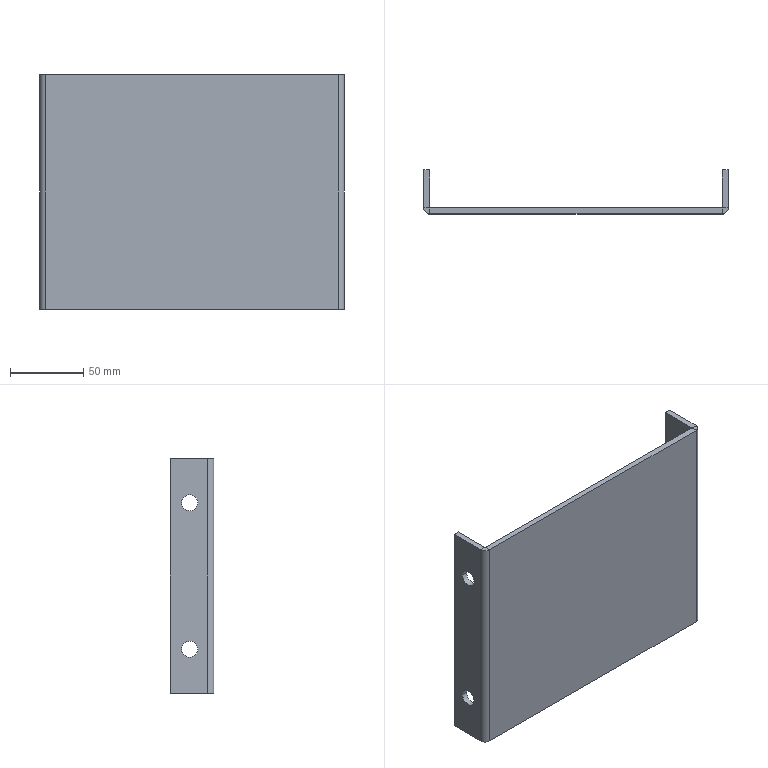Part | SolidWorks | features FlatPattern 1, ICE 1, SMBaseFlange 1, SheetMetal 1 | 1 solid | 30 faces | box 208 x 30 x 160 mm | volume 163671 mm3 | plane 18 | cylinder 12 | commonest cylinder face diameters 11 x8 0.4 x2 8.4 x2
STEP:
#1=CARTESIAN_POINT('',(100.,22.,50.));
#2=VERTEX_POINT('',#1);
#3=CARTESIAN_POINT('',(100.,11.,50.));
#4=VERTEX_POINT('',#3);
#5=CARTESIAN_POINT('',(100.,16.5,50.));
#6=DIRECTION('',(-1.,0.,0.));
#7=DIRECTION('',(0.,-1.,0.));
#8=AXIS2_PLACEMENT_3D('',#5,#6,#7);
#9=CIRCLE('',#8,5.5);
#10=EDGE_CURVE('',#2,#4,#9,.T.);
#11=ORIENTED_EDGE('',*,*,#10,.T.);
#12=CARTESIAN_POINT('',(104.,11.,50.));
#13=VERTEX_POINT('',#12);
#14=CARTESIAN_POINT('',(-104.,11.,50.));
#15=DIRECTION('',(1.,0.,0.));
#16=VECTOR('',#15,1000.);
#17=LINE('',#14,#16);
#18=EDGE_CURVE('',#4,#13,#17,.T.);
#19=ORIENTED_EDGE('',*,*,#18,.T.);
#20=CARTESIAN_POINT('',(104.,22.,50.));
#21=VERTEX_POINT('',#20);
#22=CARTESIAN_POINT('',(104.,16.5,50.));
#23=DIRECTION('',(-1.,0.,0.));
#24=DIRECTION('',(0.,-1.,0.));
#25=AXIS2_PLACEMENT_3D('',#22,#23,#24);
#26=CIRCLE('',#25,5.5);
#27=EDGE_CURVE('',#21,#13,#26,.T.);
#28=ORIENTED_EDGE('',*,*,#27,.F.);
#29=CARTESIAN_POINT('',(-104.,22.,50.));
#30=DIRECTION('',(1.,0.,0.));
#31=VECTOR('',#30,1000.);
#32=LINE('',#29,#31);
#33=EDGE_CURVE('',#2,#21,#32,.T.);
#34=ORIENTED_EDGE('',*,*,#33,.F.);
#35=EDGE_LOOP('',(#11,#19,#28,#34));
#36=FACE_OUTER_BOUND('',#35,.T.);
#37=CARTESIAN_POINT('',(-104.,16.5,50.));
#38=DIRECTION('',(1.,0.,0.));
#39=DIRECTION('',(0.,1.,0.));
#40=AXIS2_PLACEMENT_3D('',#37,#38,#39);
#41=CYLINDRICAL_SURFACE('',#40,5.5);
#42=ADVANCED_FACE('',(#36),#41,.F.);
#43=CARTESIAN_POINT('',(100.,22.,-50.));
#44=VERTEX_POINT('',#43);
#45=CARTESIAN_POINT('',(100.,11.,-50.));
#46=VERTEX_POINT('',#45);
#47=CARTESIAN_POINT('',(100.,16.5,-50.));
#48=DIRECTION('',(-1.,0.,0.));
#49=DIRECTION('',(0.,-1.,0.));
#50=AXIS2_PLACEMENT_3D('',#47,#48,#49);
#51=CIRCLE('',#50,5.5);
#52=EDGE_CURVE('',#44,#46,#51,.T.);
#53=ORIENTED_EDGE('',*,*,#52,.T.);
#54=CARTESIAN_POINT('',(104.,11.,-50.));
#55=VERTEX_POINT('',#54);
#56=CARTESIAN_POINT('',(-104.,11.,-50.));
#57=DIRECTION('',(1.,0.,0.));
#58=VECTOR('',#57,1000.);
#59=LINE('',#56,#58);
#60=EDGE_CURVE('',#46,#55,#59,.T.);
#61=ORIENTED_EDGE('',*,*,#60,.T.);
#62=CARTESIAN_POINT('',(104.,22.,-50.));
#63=VERTEX_POINT('',#62);
#64=CARTESIAN_POINT('',(104.,16.5,-50.));
#65=DIRECTION('',(-1.,0.,0.));
#66=DIRECTION('',(0.,-1.,0.));
#67=AXIS2_PLACEMENT_3D('',#64,#65,#66);
#68=CIRCLE('',#67,5.5);
#69=EDGE_CURVE('',#63,#55,#68,.T.);
#70=ORIENTED_EDGE('',*,*,#69,.F.);
#71=CARTESIAN_POINT('',(-104.,22.,-50.));
#72=DIRECTION('',(1.,0.,0.));
#73=VECTOR('',#72,1000.);
#74=LINE('',#71,#73);
#75=EDGE_CURVE('',#44,#63,#74,.T.);
#76=ORIENTED_EDGE('',*,*,#75,.F.);
#77=EDGE_LOOP('',(#53,#61,#70,#76));
#78=FACE_OUTER_BOUND('',#77,.T.);
#79=CARTESIAN_POINT('',(-104.,16.5,-50.));
#80=DIRECTION('',(1.,0.,0.));
#81=DIRECTION('',(0.,1.,0.));
#82=AXIS2_PLACEMENT_3D('',#79,#80,#81);
#83=CYLINDRICAL_SURFACE('',#82,5.5);
#84=ADVANCED_FACE('',(#78),#83,.F.);
#85=CARTESIAN_POINT('',(-104.,11.,50.));
#86=VERTEX_POINT('',#85);
#87=CARTESIAN_POINT('',(-104.,22.,50.));
#88=VERTEX_POINT('',#87);
#89=CARTESIAN_POINT('',(-104.,16.5,50.));
#90=DIRECTION('',(1.,0.,0.));
#91=DIRECTION('',(0.,1.,0.));
#92=AXIS2_PLACEMENT_3D('',#89,#90,#91);
#93=CIRCLE('',#92,5.5);
#94=EDGE_CURVE('',#86,#88,#93,.T.);
#95=ORIENTED_EDGE('',*,*,#94,.F.);
#96=CARTESIAN_POINT('',(-100.,11.,50.));
#97=VERTEX_POINT('',#96);
#98=CARTESIAN_POINT('',(-104.,11.,50.));
#99=DIRECTION('',(1.,0.,0.));
#100=VECTOR('',#99,1000.);
#101=LINE('',#98,#100);
#102=EDGE_CURVE('',#86,#97,#101,.T.);
#103=ORIENTED_EDGE('',*,*,#102,.T.);
#104=CARTESIAN_POINT('',(-100.,22.,50.));
#105=VERTEX_POINT('',#104);
#106=CARTESIAN_POINT('',(-100.,16.5,50.));
#107=DIRECTION('',(1.,0.,0.));
#108=DIRECTION('',(0.,1.,0.));
#109=AXIS2_PLACEMENT_3D('',#106,#107,#108);
#110=CIRCLE('',#109,5.5);
#111=EDGE_CURVE('',#97,#105,#110,.T.);
#112=ORIENTED_EDGE('',*,*,#111,.T.);
#113=CARTESIAN_POINT('',(-104.,22.,50.));
#114=DIRECTION('',(1.,0.,0.));
#115=VECTOR('',#114,1000.);
#116=LINE('',#113,#115);
#117=EDGE_CURVE('',#88,#105,#116,.T.);
#118=ORIENTED_EDGE('',*,*,#117,.F.);
#119=EDGE_LOOP('',(#95,#103,#112,#118));
#120=FACE_OUTER_BOUND('',#119,.T.);
#121=CARTESIAN_POINT('',(-104.,16.5,50.));
#122=DIRECTION('',(1.,0.,0.));
#123=DIRECTION('',(0.,1.,0.));
#124=AXIS2_PLACEMENT_3D('',#121,#122,#123);
#125=CYLINDRICAL_SURFACE('',#124,5.5);
#126=ADVANCED_FACE('',(#120),#125,.F.);
#127=CARTESIAN_POINT('',(-104.,11.,-50.));
#128=VERTEX_POINT('',#127);
#129=CARTESIAN_POINT('',(-104.,22.,-50.));
#130=VERTEX_POINT('',#129);
#131=CARTESIAN_POINT('',(-104.,16.5,-50.));
#132=DIRECTION('',(1.,0.,0.));
#133=DIRECTION('',(0.,1.,0.));
#134=AXIS2_PLACEMENT_3D('',#131,#132,#133);
#135=CIRCLE('',#134,5.5);
#136=EDGE_CURVE('',#128,#130,#135,.T.);
#137=ORIENTED_EDGE('',*,*,#136,.F.);
#138=CARTESIAN_POINT('',(-100.,11.,-50.));
#139=VERTEX_POINT('',#138);
#140=CARTESIAN_POINT('',(-104.,11.,-50.));
#141=DIRECTION('',(1.,0.,0.));
#142=VECTOR('',#141,1000.);
#143=LINE('',#140,#142);
#144=EDGE_CURVE('',#128,#139,#143,.T.);
#145=ORIENTED_EDGE('',*,*,#144,.T.);
#146=CARTESIAN_POINT('',(-100.,22.,-50.));
#147=VERTEX_POINT('',#146);
#148=CARTESIAN_POINT('',(-100.,16.5,-50.));
#149=DIRECTION('',(1.,0.,0.));
#150=DIRECTION('',(0.,1.,0.));
#151=AXIS2_PLACEMENT_3D('',#148,#149,#150);
#152=CIRCLE('',#151,5.5);
#153=EDGE_CURVE('',#139,#147,#152,.T.);
#154=ORIENTED_EDGE('',*,*,#153,.T.);
#155=CARTESIAN_POINT('',(-104.,22.,-50.));
#156=DIRECTION('',(1.,0.,0.));
#157=VECTOR('',#156,1000.);
#158=LINE('',#155,#157);
#159=EDGE_CURVE('',#130,#147,#158,.T.);
#160=ORIENTED_EDGE('',*,*,#159,.F.);
#161=EDGE_LOOP('',(#137,#145,#154,#160));
#162=FACE_OUTER_BOUND('',#161,.T.);
#163=CARTESIAN_POINT('',(-104.,16.5,-50.));
#164=DIRECTION('',(1.,0.,0.));
#165=DIRECTION('',(0.,1.,0.));
#166=AXIS2_PLACEMENT_3D('',#163,#164,#165);
#167=CYLINDRICAL_SURFACE('',#166,5.5);
#168=ADVANCED_FACE('',(#162),#167,.F.);
#169=CARTESIAN_POINT('',(-104.,4.2,80.));
#170=VERTEX_POINT('',#169);
#171=CARTESIAN_POINT('',(-100.,4.2,80.));
#172=VERTEX_POINT('',#171);
#173=CARTESIAN_POINT('',(-104.,4.2,80.));
#174=DIRECTION('',(1.,0.,0.));
#175=VECTOR('',#174,1000.);
#176=LINE('',#173,#175);
#177=EDGE_CURVE('',#170,#172,#176,.T.);
#178=ORIENTED_EDGE('',*,*,#177,.F.);
#179=CARTESIAN_POINT('',(-99.8,0.,80.));
#180=VERTEX_POINT('',#179);
#181=CARTESIAN_POINT('',(-99.8,4.2,80.));
#182=DIRECTION('',(0.,0.,1.));
#183=DIRECTION('',(-1.,0.,0.));
#184=AXIS2_PLACEMENT_3D('',#181,#182,#183);
#185=CIRCLE('',#184,4.2);
#186=EDGE_CURVE('',#170,#180,#185,.T.);
#187=ORIENTED_EDGE('',*,*,#186,.T.);
#188=CARTESIAN_POINT('',(-99.8,4.,80.));
#189=VERTEX_POINT('',#188);
#190=CARTESIAN_POINT('',(-99.8,4.,80.));
#191=DIRECTION('',(0.,-1.,0.));
#192=VECTOR('',#191,1000.);
#193=LINE('',#190,#192);
#194=EDGE_CURVE('',#189,#180,#193,.T.);
#195=ORIENTED_EDGE('',*,*,#194,.F.);
#196=CARTESIAN_POINT('',(-99.8,4.2,80.));
#197=DIRECTION('',(0.,0.,1.));
#198=DIRECTION('',(1.,0.,0.));
#199=AXIS2_PLACEMENT_3D('',#196,#197,#198);
#200=CIRCLE('',#199,0.2);
#201=EDGE_CURVE('',#172,#189,#200,.T.);
#202=ORIENTED_EDGE('',*,*,#201,.F.);
#203=EDGE_LOOP('',(#178,#187,#195,#202));
#204=FACE_OUTER_BOUND('',#203,.T.);
#205=CARTESIAN_POINT('',(-104.,4.2,80.));
#206=DIRECTION('',(0.,0.,1.));
#207=DIRECTION('',(1.,0.,0.));
#208=AXIS2_PLACEMENT_3D('',#205,#206,#207);
#209=PLANE('',#208);
#210=ADVANCED_FACE('',(#204),#209,.T.);
#211=CARTESIAN_POINT('',(-104.,30.,80.));
#212=VERTEX_POINT('',#211);
#213=CARTESIAN_POINT('',(-104.,30.,80.));
#214=DIRECTION('',(0.,-1.,0.));
#215=VECTOR('',#214,1000.);
#216=LINE('',#213,#215);
#217=EDGE_CURVE('',#212,#170,#216,.T.);
#218=ORIENTED_EDGE('',*,*,#217,.T.);
#219=ORIENTED_EDGE('',*,*,#177,.T.);
#220=CARTESIAN_POINT('',(-100.,30.,80.));
#221=VERTEX_POINT('',#220);
#222=CARTESIAN_POINT('',(-100.,30.,80.));
#223=DIRECTION('',(0.,-1.,0.));
#224=VECTOR('',#223,1000.);
#225=LINE('',#222,#224);
#226=EDGE_CURVE('',#221,#172,#225,.T.);
#227=ORIENTED_EDGE('',*,*,#226,.F.);
#228=CARTESIAN_POINT('',(-104.,30.,80.));
#229=DIRECTION('',(1.,0.,0.));
#230=VECTOR('',#229,1000.);
#231=LINE('',#228,#230);
#232=EDGE_CURVE('',#212,#221,#231,.T.);
#233=ORIENTED_EDGE('',*,*,#232,.F.);
#234=EDGE_LOOP('',(#218,#219,#227,#233));
#235=FACE_OUTER_BOUND('',#234,.T.);
#236=CARTESIAN_POINT('',(-99.8,4.,80.));
#237=DIRECTION('',(0.,0.,1.));
#238=DIRECTION('',(1.,0.,0.));
#239=AXIS2_PLACEMENT_3D('',#236,#237,#238);
#240=PLANE('',#239);
#241=ADVANCED_FACE('',(#235),#240,.T.);
#242=CARTESIAN_POINT('',(-99.8,0.,-80.));
#243=VERTEX_POINT('',#242);
#244=CARTESIAN_POINT('',(-99.8,4.,-80.));
#245=VERTEX_POINT('',#244);
#246=CARTESIAN_POINT('',(-99.8,0.,-80.));
#247=DIRECTION('',(0.,1.,0.));
#248=VECTOR('',#247,1000.);
#249=LINE('',#246,#248);
#250=EDGE_CURVE('',#243,#245,#249,.T.);
#251=ORIENTED_EDGE('',*,*,#250,.F.);
#252=CARTESIAN_POINT('',(-104.,4.2,-80.));
#253=VERTEX_POINT('',#252);
#254=CARTESIAN_POINT('',(-99.8,4.2,-80.));
#255=DIRECTION('',(0.,0.,1.));
#256=DIRECTION('',(-1.,0.,0.));
#257=AXIS2_PLACEMENT_3D('',#254,#255,#256);
#258=CIRCLE('',#257,4.2);
#259=EDGE_CURVE('',#253,#243,#258,.T.);
#260=ORIENTED_EDGE('',*,*,#259,.F.);
#261=CARTESIAN_POINT('',(-100.,4.2,-80.));
#262=VERTEX_POINT('',#261);
#263=CARTESIAN_POINT('',(-100.,4.2,-80.));
#264=DIRECTION('',(-1.,0.,0.));
#265=VECTOR('',#264,1000.);
#266=LINE('',#263,#265);
#267=EDGE_CURVE('',#262,#253,#266,.T.);
#268=ORIENTED_EDGE('',*,*,#267,.F.);
#269=CARTESIAN_POINT('',(-99.8,4.2,-80.));
#270=DIRECTION('',(0.,0.,1.));
#271=DIRECTION('',(1.,0.,0.));
#272=AXIS2_PLACEMENT_3D('',#269,#270,#271);
#273=CIRCLE('',#272,0.2);
#274=EDGE_CURVE('',#262,#245,#273,.T.);
#275=ORIENTED_EDGE('',*,*,#274,.T.);
#276=EDGE_LOOP('',(#251,#260,#268,#275));
#277=FACE_OUTER_BOUND('',#276,.T.);
#278=CARTESIAN_POINT('',(-99.8,0.,-80.));
#279=DIRECTION('',(0.,0.,-1.));
#280=DIRECTION('',(-1.,0.,0.));
#281=AXIS2_PLACEMENT_3D('',#278,#279,#280);
#282=PLANE('',#281);
#283=ADVANCED_FACE('',(#277),#282,.T.);
#284=CARTESIAN_POINT('',(99.8,0.,-80.));
#285=VERTEX_POINT('',#284);
#286=CARTESIAN_POINT('',(-104.,0.,-80.));
#287=DIRECTION('',(1.,0.,0.));
#288=VECTOR('',#287,1000.);
#289=LINE('',#286,#288);
#290=EDGE_CURVE('',#243,#285,#289,.T.);
#291=ORIENTED_EDGE('',*,*,#290,.F.);
#292=ORIENTED_EDGE('',*,*,#250,.T.);
#293=CARTESIAN_POINT('',(99.8,4.,-80.));
#294=VERTEX_POINT('',#293);
#295=CARTESIAN_POINT('',(-104.,4.,-80.));
#296=DIRECTION('',(1.,0.,0.));
#297=VECTOR('',#296,1000.);
#298=LINE('',#295,#297);
#299=EDGE_CURVE('',#245,#294,#298,.T.);
#300=ORIENTED_EDGE('',*,*,#299,.T.);
#301=CARTESIAN_POINT('',(99.8,4.,-80.));
#302=DIRECTION('',(0.,-1.,0.));
#303=VECTOR('',#302,1000.);
#304=LINE('',#301,#303);
#305=EDGE_CURVE('',#294,#285,#304,.T.);
#306=ORIENTED_EDGE('',*,*,#305,.T.);
#307=EDGE_LOOP('',(#291,#292,#300,#306));
#308=FACE_OUTER_BOUND('',#307,.T.);
#309=CARTESIAN_POINT('',(-100.,4.2,-80.));
#310=DIRECTION('',(0.,0.,-1.));
#311=DIRECTION('',(-1.,0.,0.));
#312=AXIS2_PLACEMENT_3D('',#309,#310,#311);
#313=PLANE('',#312);
#314=ADVANCED_FACE('',(#308),#313,.T.);
#315=CARTESIAN_POINT('',(99.8,0.,80.));
#316=VERTEX_POINT('',#315);
#317=CARTESIAN_POINT('',(99.8,4.,80.));
#318=VERTEX_POINT('',#317);
#319=CARTESIAN_POINT('',(99.8,0.,80.));
#320=DIRECTION('',(0.,1.,0.));
#321=VECTOR('',#320,1000.);
#322=LINE('',#319,#321);
#323=EDGE_CURVE('',#316,#318,#322,.T.);
#324=ORIENTED_EDGE('',*,*,#323,.F.);
#325=CARTESIAN_POINT('',(104.,4.2,80.));
#326=VERTEX_POINT('',#325);
#327=CARTESIAN_POINT('',(99.8,4.2,80.));
#328=DIRECTION('',(0.,0.,1.));
#329=DIRECTION('',(-1.,0.,0.));
#330=AXIS2_PLACEMENT_3D('',#327,#328,#329);
#331=CIRCLE('',#330,4.2);
#332=EDGE_CURVE('',#316,#326,#331,.T.);
#333=ORIENTED_EDGE('',*,*,#332,.T.);
#334=CARTESIAN_POINT('',(100.,4.2,80.));
#335=VERTEX_POINT('',#334);
#336=CARTESIAN_POINT('',(100.,4.2,80.));
#337=DIRECTION('',(1.,0.,0.));
#338=VECTOR('',#337,1000.);
#339=LINE('',#336,#338);
#340=EDGE_CURVE('',#335,#326,#339,.T.);
#341=ORIENTED_EDGE('',*,*,#340,.F.);
#342=CARTESIAN_POINT('',(99.8,4.2,80.));
#343=DIRECTION('',(0.,0.,1.));
#344=DIRECTION('',(1.,0.,0.));
#345=AXIS2_PLACEMENT_3D('',#342,#343,#344);
#346=CIRCLE('',#345,0.2);
#347=EDGE_CURVE('',#318,#335,#346,.T.);
#348=ORIENTED_EDGE('',*,*,#347,.F.);
#349=EDGE_LOOP('',(#324,#333,#341,#348));
#350=FACE_OUTER_BOUND('',#349,.T.);
#351=CARTESIAN_POINT('',(99.8,0.,80.));
#352=DIRECTION('',(0.,0.,1.));
#353=DIRECTION('',(1.,0.,0.));
#354=AXIS2_PLACEMENT_3D('',#351,#352,#353);
#355=PLANE('',#354);
#356=ADVANCED_FACE('',(#350),#355,.T.);
#357=CARTESIAN_POINT('',(-104.,0.,80.));
#358=DIRECTION('',(1.,0.,0.));
#359=VECTOR('',#358,1000.);
#360=LINE('',#357,#359);
#361=EDGE_CURVE('',#180,#316,#360,.T.);
#362=ORIENTED_EDGE('',*,*,#361,.T.);
#363=ORIENTED_EDGE('',*,*,#323,.T.);
#364=CARTESIAN_POINT('',(-104.,4.,80.));
#365=DIRECTION('',(1.,0.,0.));
#366=VECTOR('',#365,1000.);
#367=LINE('',#364,#366);
#368=EDGE_CURVE('',#189,#318,#367,.T.);
#369=ORIENTED_EDGE('',*,*,#368,.F.);
#370=ORIENTED_EDGE('',*,*,#194,.T.);
#371=EDGE_LOOP('',(#362,#363,#369,#370));
#372=FACE_OUTER_BOUND('',#371,.T.);
#373=CARTESIAN_POINT('',(100.,4.2,80.));
#374=DIRECTION('',(0.,0.,1.));
#375=DIRECTION('',(1.,0.,0.));
#376=AXIS2_PLACEMENT_3D('',#373,#374,#375);
#377=PLANE('',#376);
#378=ADVANCED_FACE('',(#372),#377,.T.);
#379=CARTESIAN_POINT('',(104.,4.2,-80.));
#380=VERTEX_POINT('',#379);
#381=CARTESIAN_POINT('',(100.,4.2,-80.));
#382=VERTEX_POINT('',#381);
#383=CARTESIAN_POINT('',(104.,4.2,-80.));
#384=DIRECTION('',(-1.,0.,0.));
#385=VECTOR('',#384,1000.);
#386=LINE('',#383,#385);
#387=EDGE_CURVE('',#380,#382,#386,.T.);
#388=ORIENTED_EDGE('',*,*,#387,.F.);
#389=CARTESIAN_POINT('',(99.8,4.2,-80.));
#390=DIRECTION('',(0.,0.,1.));
#391=DIRECTION('',(-1.,0.,0.));
#392=AXIS2_PLACEMENT_3D('',#389,#390,#391);
#393=CIRCLE('',#392,4.2);
#394=EDGE_CURVE('',#285,#380,#393,.T.);
#395=ORIENTED_EDGE('',*,*,#394,.F.);
#396=ORIENTED_EDGE('',*,*,#305,.F.);
#397=CARTESIAN_POINT('',(99.8,4.2,-80.));
#398=DIRECTION('',(0.,0.,1.));
#399=DIRECTION('',(1.,0.,0.));
#400=AXIS2_PLACEMENT_3D('',#397,#398,#399);
#401=CIRCLE('',#400,0.2);
#402=EDGE_CURVE('',#294,#382,#401,.T.);
#403=ORIENTED_EDGE('',*,*,#402,.T.);
#404=EDGE_LOOP('',(#388,#395,#396,#403));
#405=FACE_OUTER_BOUND('',#404,.T.);
#406=CARTESIAN_POINT('',(104.,4.2,-80.));
#407=DIRECTION('',(0.,0.,-1.));
#408=DIRECTION('',(-1.,0.,0.));
#409=AXIS2_PLACEMENT_3D('',#406,#407,#408);
#410=PLANE('',#409);
#411=ADVANCED_FACE('',(#405),#410,.T.);
#412=CARTESIAN_POINT('',(104.,30.,-80.));
#413=VERTEX_POINT('',#412);
#414=CARTESIAN_POINT('',(104.,0.,-80.));
#415=DIRECTION('',(0.,1.,0.));
#416=VECTOR('',#415,1000.);
#417=LINE('',#414,#416);
#418=EDGE_CURVE('',#380,#413,#417,.T.);
#419=ORIENTED_EDGE('',*,*,#418,.F.);
#420=ORIENTED_EDGE('',*,*,#387,.T.);
#421=CARTESIAN_POINT('',(100.,30.,-80.));
#422=VERTEX_POINT('',#421);
#423=CARTESIAN_POINT('',(100.,0.,-80.));
#424=DIRECTION('',(0.,1.,0.));
#425=VECTOR('',#424,1000.);
#426=LINE('',#423,#425);
#427=EDGE_CURVE('',#382,#422,#426,.T.);
#428=ORIENTED_EDGE('',*,*,#427,.T.);
#429=CARTESIAN_POINT('',(100.,30.,-80.));
#430=DIRECTION('',(1.,0.,0.));
#431=VECTOR('',#430,1000.);
#432=LINE('',#429,#431);
#433=EDGE_CURVE('',#422,#413,#432,.T.);
#434=ORIENTED_EDGE('',*,*,#433,.T.);
#435=EDGE_LOOP('',(#419,#420,#428,#434));
#436=FACE_OUTER_BOUND('',#435,.T.);
#437=CARTESIAN_POINT('',(99.8,4.,-80.));
#438=DIRECTION('',(0.,0.,-1.));
#439=DIRECTION('',(-1.,0.,0.));
#440=AXIS2_PLACEMENT_3D('',#437,#438,#439);
#441=PLANE('',#440);
#442=ADVANCED_FACE('',(#436),#441,.T.);
#443=ORIENTED_EDGE('',*,*,#27,.T.);
#444=CARTESIAN_POINT('',(104.,16.5,50.));
#445=DIRECTION('',(-1.,0.,0.));
#446=DIRECTION('',(0.,-1.,0.));
#447=AXIS2_PLACEMENT_3D('',#444,#445,#446);
#448=CIRCLE('',#447,5.5);
#449=EDGE_CURVE('',#13,#21,#448,.T.);
#450=ORIENTED_EDGE('',*,*,#449,.T.);
#451=EDGE_LOOP('',(#443,#450));
#452=FACE_BOUND('',#451,.T.);
#453=ORIENTED_EDGE('',*,*,#69,.T.);
#454=CARTESIAN_POINT('',(104.,16.5,-50.));
#455=DIRECTION('',(-1.,0.,0.));
#456=DIRECTION('',(0.,-1.,0.));
#457=AXIS2_PLACEMENT_3D('',#454,#455,#456);
#458=CIRCLE('',#457,5.5);
#459=EDGE_CURVE('',#55,#63,#458,.T.);
#460=ORIENTED_EDGE('',*,*,#459,.T.);
#461=EDGE_LOOP('',(#453,#460));
#462=FACE_BOUND('',#461,.T.);
#463=ORIENTED_EDGE('',*,*,#418,.T.);
#464=CARTESIAN_POINT('',(104.,30.,80.));
#465=VERTEX_POINT('',#464);
#466=CARTESIAN_POINT('',(104.,30.,80.));
#467=DIRECTION('',(0.,0.,-1.));
#468=VECTOR('',#467,1000.);
#469=LINE('',#466,#468);
#470=EDGE_CURVE('',#465,#413,#469,.T.);
#471=ORIENTED_EDGE('',*,*,#470,.F.);
#472=CARTESIAN_POINT('',(104.,0.,80.));
#473=DIRECTION('',(0.,1.,0.));
#474=VECTOR('',#473,1000.);
#475=LINE('',#472,#474);
#476=EDGE_CURVE('',#326,#465,#475,.T.);
#477=ORIENTED_EDGE('',*,*,#476,.F.);
#478=CARTESIAN_POINT('',(104.,4.2,80.));
#479=DIRECTION('',(0.,0.,-1.));
#480=VECTOR('',#479,1000.);
#481=LINE('',#478,#480);
#482=EDGE_CURVE('',#326,#380,#481,.T.);
#483=ORIENTED_EDGE('',*,*,#482,.T.);
#484=EDGE_LOOP('',(#463,#471,#477,#483));
#485=FACE_OUTER_BOUND('',#484,.T.);
#486=CARTESIAN_POINT('',(104.,0.,80.));
#487=DIRECTION('',(-1.,0.,0.));
#488=DIRECTION('',(0.,-1.,0.));
#489=AXIS2_PLACEMENT_3D('',#486,#487,#488);
#490=PLANE('',#489);
#491=ADVANCED_FACE('',(#452,#462,#485),#490,.F.);
#492=ORIENTED_EDGE('',*,*,#433,.F.);
#493=CARTESIAN_POINT('',(100.,30.,80.));
#494=VERTEX_POINT('',#493);
#495=CARTESIAN_POINT('',(100.,30.,80.));
#496=DIRECTION('',(0.,0.,-1.));
#497=VECTOR('',#496,1000.);
#498=LINE('',#495,#497);
#499=EDGE_CURVE('',#494,#422,#498,.T.);
#500=ORIENTED_EDGE('',*,*,#499,.F.);
#501=CARTESIAN_POINT('',(100.,30.,80.));
#502=DIRECTION('',(1.,0.,0.));
#503=VECTOR('',#502,1000.);
#504=LINE('',#501,#503);
#505=EDGE_CURVE('',#494,#465,#504,.T.);
#506=ORIENTED_EDGE('',*,*,#505,.T.);
#507=ORIENTED_EDGE('',*,*,#470,.T.);
#508=EDGE_LOOP('',(#492,#500,#506,#507));
#509=FACE_OUTER_BOUND('',#508,.T.);
#510=CARTESIAN_POINT('',(100.,30.,80.));
#511=DIRECTION('',(0.,1.,0.));
#512=DIRECTION('',(-1.,0.,0.));
#513=AXIS2_PLACEMENT_3D('',#510,#511,#512);
#514=PLANE('',#513);
#515=ADVANCED_FACE('',(#509),#514,.T.);
#516=ORIENTED_EDGE('',*,*,#10,.F.);
#517=CARTESIAN_POINT('',(100.,16.5,50.));
#518=DIRECTION('',(-1.,0.,0.));
#519=DIRECTION('',(0.,-1.,0.));
#520=AXIS2_PLACEMENT_3D('',#517,#518,#519);
#521=CIRCLE('',#520,5.5);
#522=EDGE_CURVE('',#4,#2,#521,.T.);
#523=ORIENTED_EDGE('',*,*,#522,.F.);
#524=EDGE_LOOP('',(#516,#523));
#525=FACE_BOUND('',#524,.T.);
#526=ORIENTED_EDGE('',*,*,#52,.F.);
#527=CARTESIAN_POINT('',(100.,16.5,-50.));
#528=DIRECTION('',(-1.,0.,0.));
#529=DIRECTION('',(0.,-1.,0.));
#530=AXIS2_PLACEMENT_3D('',#527,#528,#529);
#531=CIRCLE('',#530,5.5);
#532=EDGE_CURVE('',#46,#44,#531,.T.);
#533=ORIENTED_EDGE('',*,*,#532,.F.);
#534=EDGE_LOOP('',(#526,#533));
#535=FACE_BOUND('',#534,.T.);
#536=ORIENTED_EDGE('',*,*,#427,.F.);
#537=CARTESIAN_POINT('',(100.,4.2,80.));
#538=DIRECTION('',(0.,0.,-1.));
#539=VECTOR('',#538,1000.);
#540=LINE('',#537,#539);
#541=EDGE_CURVE('',#335,#382,#540,.T.);
#542=ORIENTED_EDGE('',*,*,#541,.F.);
#543=CARTESIAN_POINT('',(100.,0.,80.));
#544=DIRECTION('',(0.,1.,0.));
#545=VECTOR('',#544,1000.);
#546=LINE('',#543,#545);
#547=EDGE_CURVE('',#335,#494,#546,.T.);
#548=ORIENTED_EDGE('',*,*,#547,.T.);
#549=ORIENTED_EDGE('',*,*,#499,.T.);
#550=EDGE_LOOP('',(#536,#542,#548,#549));
#551=FACE_OUTER_BOUND('',#550,.T.);
#552=CARTESIAN_POINT('',(100.,0.,80.));
#553=DIRECTION('',(-1.,0.,0.));
#554=DIRECTION('',(0.,-1.,0.));
#555=AXIS2_PLACEMENT_3D('',#552,#553,#554);
#556=PLANE('',#555);
#557=ADVANCED_FACE('',(#525,#535,#551),#556,.T.);
#558=ORIENTED_EDGE('',*,*,#402,.F.);
#559=CARTESIAN_POINT('',(99.8,4.,80.));
#560=DIRECTION('',(0.,0.,-1.));
#561=VECTOR('',#560,1000.);
#562=LINE('',#559,#561);
#563=EDGE_CURVE('',#318,#294,#562,.T.);
#564=ORIENTED_EDGE('',*,*,#563,.F.);
#565=ORIENTED_EDGE('',*,*,#347,.T.);
#566=ORIENTED_EDGE('',*,*,#541,.T.);
#567=EDGE_LOOP('',(#558,#564,#565,#566));
#568=FACE_OUTER_BOUND('',#567,.T.);
#569=CARTESIAN_POINT('',(99.8,4.2,80.));
#570=DIRECTION('',(0.,0.,-1.));
#571=DIRECTION('',(-1.,0.,0.));
#572=AXIS2_PLACEMENT_3D('',#569,#570,#571);
#573=CYLINDRICAL_SURFACE('',#572,0.2);
#574=ADVANCED_FACE('',(#568),#573,.F.);
#575=ORIENTED_EDGE('',*,*,#299,.F.);
#576=CARTESIAN_POINT('',(-99.8,4.,80.));
#577=DIRECTION('',(0.,0.,-1.));
#578=VECTOR('',#577,1000.);
#579=LINE('',#576,#578);
#580=EDGE_CURVE('',#189,#245,#579,.T.);
#581=ORIENTED_EDGE('',*,*,#580,.F.);
#582=ORIENTED_EDGE('',*,*,#368,.T.);
#583=ORIENTED_EDGE('',*,*,#563,.T.);
#584=EDGE_LOOP('',(#575,#581,#582,#583));
#585=FACE_OUTER_BOUND('',#584,.T.);
#586=CARTESIAN_POINT('',(-104.,4.,80.));
#587=DIRECTION('',(0.,1.,0.));
#588=DIRECTION('',(0.,0.,1.));
#589=AXIS2_PLACEMENT_3D('',#586,#587,#588);
#590=PLANE('',#589);
#591=ADVANCED_FACE('',(#585),#590,.T.);
#592=ORIENTED_EDGE('',*,*,#274,.F.);
#593=CARTESIAN_POINT('',(-100.,4.2,80.));
#594=DIRECTION('',(0.,0.,-1.));
#595=VECTOR('',#594,1000.);
#596=LINE('',#593,#595);
#597=EDGE_CURVE('',#172,#262,#596,.T.);
#598=ORIENTED_EDGE('',*,*,#597,.F.);
#599=ORIENTED_EDGE('',*,*,#201,.T.);
#600=ORIENTED_EDGE('',*,*,#580,.T.);
#601=EDGE_LOOP('',(#592,#598,#599,#600));
#602=FACE_OUTER_BOUND('',#601,.T.);
#603=CARTESIAN_POINT('',(-99.8,4.2,80.));
#604=DIRECTION('',(0.,0.,-1.));
#605=DIRECTION('',(-1.,0.,0.));
#606=AXIS2_PLACEMENT_3D('',#603,#604,#605);
#607=CYLINDRICAL_SURFACE('',#606,0.2);
#608=ADVANCED_FACE('',(#602),#607,.F.);
#609=CARTESIAN_POINT('',(-100.,16.5,50.));
#610=DIRECTION('',(1.,0.,0.));
#611=DIRECTION('',(0.,1.,0.));
#612=AXIS2_PLACEMENT_3D('',#609,#610,#611);
#613=CIRCLE('',#612,5.5);
#614=EDGE_CURVE('',#105,#97,#613,.T.);
#615=ORIENTED_EDGE('',*,*,#614,.F.);
#616=ORIENTED_EDGE('',*,*,#111,.F.);
#617=EDGE_LOOP('',(#615,#616));
#618=FACE_BOUND('',#617,.T.);
#619=CARTESIAN_POINT('',(-100.,16.5,-50.));
#620=DIRECTION('',(1.,0.,0.));
#621=DIRECTION('',(0.,1.,0.));
#622=AXIS2_PLACEMENT_3D('',#619,#620,#621);
#623=CIRCLE('',#622,5.5);
#624=EDGE_CURVE('',#147,#139,#623,.T.);
#625=ORIENTED_EDGE('',*,*,#624,.F.);
#626=ORIENTED_EDGE('',*,*,#153,.F.);
#627=EDGE_LOOP('',(#625,#626));
#628=FACE_BOUND('',#627,.T.);
#629=CARTESIAN_POINT('',(-100.,30.,-80.));
#630=VERTEX_POINT('',#629);
#631=CARTESIAN_POINT('',(-100.,30.,-80.));
#632=DIRECTION('',(0.,-1.,0.));
#633=VECTOR('',#632,1000.);
#634=LINE('',#631,#633);
#635=EDGE_CURVE('',#630,#262,#634,.T.);
#636=ORIENTED_EDGE('',*,*,#635,.F.);
#637=CARTESIAN_POINT('',(-100.,30.,80.));
#638=DIRECTION('',(0.,0.,-1.));
#639=VECTOR('',#638,1000.);
#640=LINE('',#637,#639);
#641=EDGE_CURVE('',#221,#630,#640,.T.);
#642=ORIENTED_EDGE('',*,*,#641,.F.);
#643=ORIENTED_EDGE('',*,*,#226,.T.);
#644=ORIENTED_EDGE('',*,*,#597,.T.);
#645=EDGE_LOOP('',(#636,#642,#643,#644));
#646=FACE_OUTER_BOUND('',#645,.T.);
#647=CARTESIAN_POINT('',(-100.,30.,80.));
#648=DIRECTION('',(1.,0.,0.));
#649=DIRECTION('',(0.,1.,0.));
#650=AXIS2_PLACEMENT_3D('',#647,#648,#649);
#651=PLANE('',#650);
#652=ADVANCED_FACE('',(#618,#628,#646),#651,.T.);
#653=CARTESIAN_POINT('',(-104.,30.,-80.));
#654=VERTEX_POINT('',#653);
#655=CARTESIAN_POINT('',(-104.,30.,-80.));
#656=DIRECTION('',(1.,0.,0.));
#657=VECTOR('',#656,1000.);
#658=LINE('',#655,#657);
#659=EDGE_CURVE('',#654,#630,#658,.T.);
#660=ORIENTED_EDGE('',*,*,#659,.F.);
#661=CARTESIAN_POINT('',(-104.,30.,80.));
#662=DIRECTION('',(0.,0.,-1.));
#663=VECTOR('',#662,1000.);
#664=LINE('',#661,#663);
#665=EDGE_CURVE('',#212,#654,#664,.T.);
#666=ORIENTED_EDGE('',*,*,#665,.F.);
#667=ORIENTED_EDGE('',*,*,#232,.T.);
#668=ORIENTED_EDGE('',*,*,#641,.T.);
#669=EDGE_LOOP('',(#660,#666,#667,#668));
#670=FACE_OUTER_BOUND('',#669,.T.);
#671=CARTESIAN_POINT('',(-104.,30.,80.));
#672=DIRECTION('',(0.,1.,0.));
#673=DIRECTION('',(-1.,0.,0.));
#674=AXIS2_PLACEMENT_3D('',#671,#672,#673);
#675=PLANE('',#674);
#676=ADVANCED_FACE('',(#670),#675,.T.);
#677=CARTESIAN_POINT('',(-104.,16.5,50.));
#678=DIRECTION('',(1.,0.,0.));
#679=DIRECTION('',(0.,1.,0.));
#680=AXIS2_PLACEMENT_3D('',#677,#678,#679);
#681=CIRCLE('',#680,5.5);
#682=EDGE_CURVE('',#88,#86,#681,.T.);
#683=ORIENTED_EDGE('',*,*,#682,.T.);
#684=ORIENTED_EDGE('',*,*,#94,.T.);
#685=EDGE_LOOP('',(#683,#684));
#686=FACE_BOUND('',#685,.T.);
#687=CARTESIAN_POINT('',(-104.,16.5,-50.));
#688=DIRECTION('',(1.,0.,0.));
#689=DIRECTION('',(0.,1.,0.));
#690=AXIS2_PLACEMENT_3D('',#687,#688,#689);
#691=CIRCLE('',#690,5.5);
#692=EDGE_CURVE('',#130,#128,#691,.T.);
#693=ORIENTED_EDGE('',*,*,#692,.T.);
#694=ORIENTED_EDGE('',*,*,#136,.T.);
#695=EDGE_LOOP('',(#693,#694));
#696=FACE_BOUND('',#695,.T.);
#697=CARTESIAN_POINT('',(-104.,30.,-80.));
#698=DIRECTION('',(0.,-1.,0.));
#699=VECTOR('',#698,1000.);
#700=LINE('',#697,#699);
#701=EDGE_CURVE('',#654,#253,#700,.T.);
#702=ORIENTED_EDGE('',*,*,#701,.T.);
#703=CARTESIAN_POINT('',(-104.,4.2,80.));
#704=DIRECTION('',(0.,0.,-1.));
#705=VECTOR('',#704,1000.);
#706=LINE('',#703,#705);
#707=EDGE_CURVE('',#170,#253,#706,.T.);
#708=ORIENTED_EDGE('',*,*,#707,.F.);
#709=ORIENTED_EDGE('',*,*,#217,.F.);
#710=ORIENTED_EDGE('',*,*,#665,.T.);
#711=EDGE_LOOP('',(#702,#708,#709,#710));
#712=FACE_OUTER_BOUND('',#711,.T.);
#713=CARTESIAN_POINT('',(-104.,30.,80.));
#714=DIRECTION('',(1.,0.,0.));
#715=DIRECTION('',(0.,1.,0.));
#716=AXIS2_PLACEMENT_3D('',#713,#714,#715);
#717=PLANE('',#716);
#718=ADVANCED_FACE('',(#686,#696,#712),#717,.F.);
#719=ORIENTED_EDGE('',*,*,#259,.T.);
#720=CARTESIAN_POINT('',(-99.8,0.,80.));
#721=DIRECTION('',(0.,0.,-1.));
#722=VECTOR('',#721,1000.);
#723=LINE('',#720,#722);
#724=EDGE_CURVE('',#180,#243,#723,.T.);
#725=ORIENTED_EDGE('',*,*,#724,.F.);
#726=ORIENTED_EDGE('',*,*,#186,.F.);
#727=ORIENTED_EDGE('',*,*,#707,.T.);
#728=EDGE_LOOP('',(#719,#725,#726,#727));
#729=FACE_OUTER_BOUND('',#728,.T.);
#730=CARTESIAN_POINT('',(-99.8,4.2,80.));
#731=DIRECTION('',(0.,0.,-1.));
#732=DIRECTION('',(-1.,0.,0.));
#733=AXIS2_PLACEMENT_3D('',#730,#731,#732);
#734=CYLINDRICAL_SURFACE('',#733,4.2);
#735=ADVANCED_FACE('',(#729),#734,.T.);
#736=ORIENTED_EDGE('',*,*,#290,.T.);
#737=CARTESIAN_POINT('',(99.8,0.,80.));
#738=DIRECTION('',(0.,0.,-1.));
#739=VECTOR('',#738,1000.);
#740=LINE('',#737,#739);
#741=EDGE_CURVE('',#316,#285,#740,.T.);
#742=ORIENTED_EDGE('',*,*,#741,.F.);
#743=ORIENTED_EDGE('',*,*,#361,.F.);
#744=ORIENTED_EDGE('',*,*,#724,.T.);
#745=EDGE_LOOP('',(#736,#742,#743,#744));
#746=FACE_OUTER_BOUND('',#745,.T.);
#747=CARTESIAN_POINT('',(-104.,0.,80.));
#748=DIRECTION('',(0.,1.,0.));
#749=DIRECTION('',(0.,0.,1.));
#750=AXIS2_PLACEMENT_3D('',#747,#748,#749);
#751=PLANE('',#750);
#752=ADVANCED_FACE('',(#746),#751,.F.);
#753=ORIENTED_EDGE('',*,*,#394,.T.);
#754=ORIENTED_EDGE('',*,*,#482,.F.);
#755=ORIENTED_EDGE('',*,*,#332,.F.);
#756=ORIENTED_EDGE('',*,*,#741,.T.);
#757=EDGE_LOOP('',(#753,#754,#755,#756));
#758=FACE_OUTER_BOUND('',#757,.T.);
#759=CARTESIAN_POINT('',(99.8,4.2,80.));
#760=DIRECTION('',(0.,0.,-1.));
#761=DIRECTION('',(-1.,0.,0.));
#762=AXIS2_PLACEMENT_3D('',#759,#760,#761);
#763=CYLINDRICAL_SURFACE('',#762,4.2);
#764=ADVANCED_FACE('',(#758),#763,.T.);
#765=ORIENTED_EDGE('',*,*,#476,.T.);
#766=ORIENTED_EDGE('',*,*,#505,.F.);
#767=ORIENTED_EDGE('',*,*,#547,.F.);
#768=ORIENTED_EDGE('',*,*,#340,.T.);
#769=EDGE_LOOP('',(#765,#766,#767,#768));
#770=FACE_OUTER_BOUND('',#769,.T.);
#771=CARTESIAN_POINT('',(99.8,4.2,80.));
#772=DIRECTION('',(0.,0.,1.));
#773=DIRECTION('',(1.,0.,0.));
#774=AXIS2_PLACEMENT_3D('',#771,#772,#773);
#775=PLANE('',#774);
#776=ADVANCED_FACE('',(#770),#775,.T.);
#777=ORIENTED_EDGE('',*,*,#635,.T.);
#778=ORIENTED_EDGE('',*,*,#267,.T.);
#779=ORIENTED_EDGE('',*,*,#701,.F.);
#780=ORIENTED_EDGE('',*,*,#659,.T.);
#781=EDGE_LOOP('',(#777,#778,#779,#780));
#782=FACE_OUTER_BOUND('',#781,.T.);
#783=CARTESIAN_POINT('',(99.8,4.2,-80.));
#784=DIRECTION('',(0.,0.,1.));
#785=DIRECTION('',(1.,0.,0.));
#786=AXIS2_PLACEMENT_3D('',#783,#784,#785);
#787=PLANE('',#786);
#788=ADVANCED_FACE('',(#782),#787,.F.);
#789=ORIENTED_EDGE('',*,*,#144,.F.);
#790=ORIENTED_EDGE('',*,*,#692,.F.);
#791=ORIENTED_EDGE('',*,*,#159,.T.);
#792=ORIENTED_EDGE('',*,*,#624,.T.);
#793=EDGE_LOOP('',(#789,#790,#791,#792));
#794=FACE_OUTER_BOUND('',#793,.T.);
#795=CARTESIAN_POINT('',(-104.,16.5,-50.));
#796=DIRECTION('',(1.,0.,0.));
#797=DIRECTION('',(0.,1.,0.));
#798=AXIS2_PLACEMENT_3D('',#795,#796,#797);
#799=CYLINDRICAL_SURFACE('',#798,5.5);
#800=ADVANCED_FACE('',(#794),#799,.F.);
#801=ORIENTED_EDGE('',*,*,#102,.F.);
#802=ORIENTED_EDGE('',*,*,#682,.F.);
#803=ORIENTED_EDGE('',*,*,#117,.T.);
#804=ORIENTED_EDGE('',*,*,#614,.T.);
#805=EDGE_LOOP('',(#801,#802,#803,#804));
#806=FACE_OUTER_BOUND('',#805,.T.);
#807=CARTESIAN_POINT('',(-104.,16.5,50.));
#808=DIRECTION('',(1.,0.,0.));
#809=DIRECTION('',(0.,1.,0.));
#810=AXIS2_PLACEMENT_3D('',#807,#808,#809);
#811=CYLINDRICAL_SURFACE('',#810,5.5);
#812=ADVANCED_FACE('',(#806),#811,.F.);
#813=ORIENTED_EDGE('',*,*,#60,.F.);
#814=ORIENTED_EDGE('',*,*,#532,.T.);
#815=ORIENTED_EDGE('',*,*,#75,.T.);
#816=ORIENTED_EDGE('',*,*,#459,.F.);
#817=EDGE_LOOP('',(#813,#814,#815,#816));
#818=FACE_OUTER_BOUND('',#817,.T.);
#819=CARTESIAN_POINT('',(-104.,16.5,-50.));
#820=DIRECTION('',(1.,0.,0.));
#821=DIRECTION('',(0.,1.,0.));
#822=AXIS2_PLACEMENT_3D('',#819,#820,#821);
#823=CYLINDRICAL_SURFACE('',#822,5.5);
#824=ADVANCED_FACE('',(#818),#823,.F.);
#825=ORIENTED_EDGE('',*,*,#18,.F.);
#826=ORIENTED_EDGE('',*,*,#522,.T.);
#827=ORIENTED_EDGE('',*,*,#33,.T.);
#828=ORIENTED_EDGE('',*,*,#449,.F.);
#829=EDGE_LOOP('',(#825,#826,#827,#828));
#830=FACE_OUTER_BOUND('',#829,.T.);
#831=CARTESIAN_POINT('',(-104.,16.5,50.));
#832=DIRECTION('',(1.,0.,0.));
#833=DIRECTION('',(0.,1.,0.));
#834=AXIS2_PLACEMENT_3D('',#831,#832,#833);
#835=CYLINDRICAL_SURFACE('',#834,5.5);
#836=ADVANCED_FACE('',(#830),#835,.F.);
#837=CLOSED_SHELL('',(#42,#84,#126,#168,#210,#241,#283,#314,#356,#378,#411,#442,#491,#515,#557,#574,#591,#608,#652,#676,#718,#735,#752,#764,#776,#788,#800,#812,#824,#836));
#838=MANIFOLD_SOLID_BREP('',#837);
#839=CARTESIAN_POINT('',(0.,0.,0.));
#840=DIRECTION('',(0.,0.,1.));
#841=DIRECTION('',(1.,0.,0.));
#842=AXIS2_PLACEMENT_3D('',#839,#840,#841);
#843=(LENGTH_UNIT()NAMED_UNIT(*)SI_UNIT(.MILLI.,.METRE.));
#844=UNCERTAINTY_MEASURE_WITH_UNIT(LENGTH_MEASURE(0.00001),#843,'','');
#845=(NAMED_UNIT(*)PLANE_ANGLE_UNIT()SI_UNIT($,.RADIAN.));
#846=(NAMED_UNIT(*)SI_UNIT($,.STERADIAN.)SOLID_ANGLE_UNIT());
#847=(GEOMETRIC_REPRESENTATION_CONTEXT(3)GLOBAL_UNCERTAINTY_ASSIGNED_CONTEXT((#844))GLOBAL_UNIT_ASSIGNED_CONTEXT((#843,#845,#846))REPRESENTATION_CONTEXT('',''));
#848=ADVANCED_BREP_SHAPE_REPRESENTATION('',(#838,#842),#847);